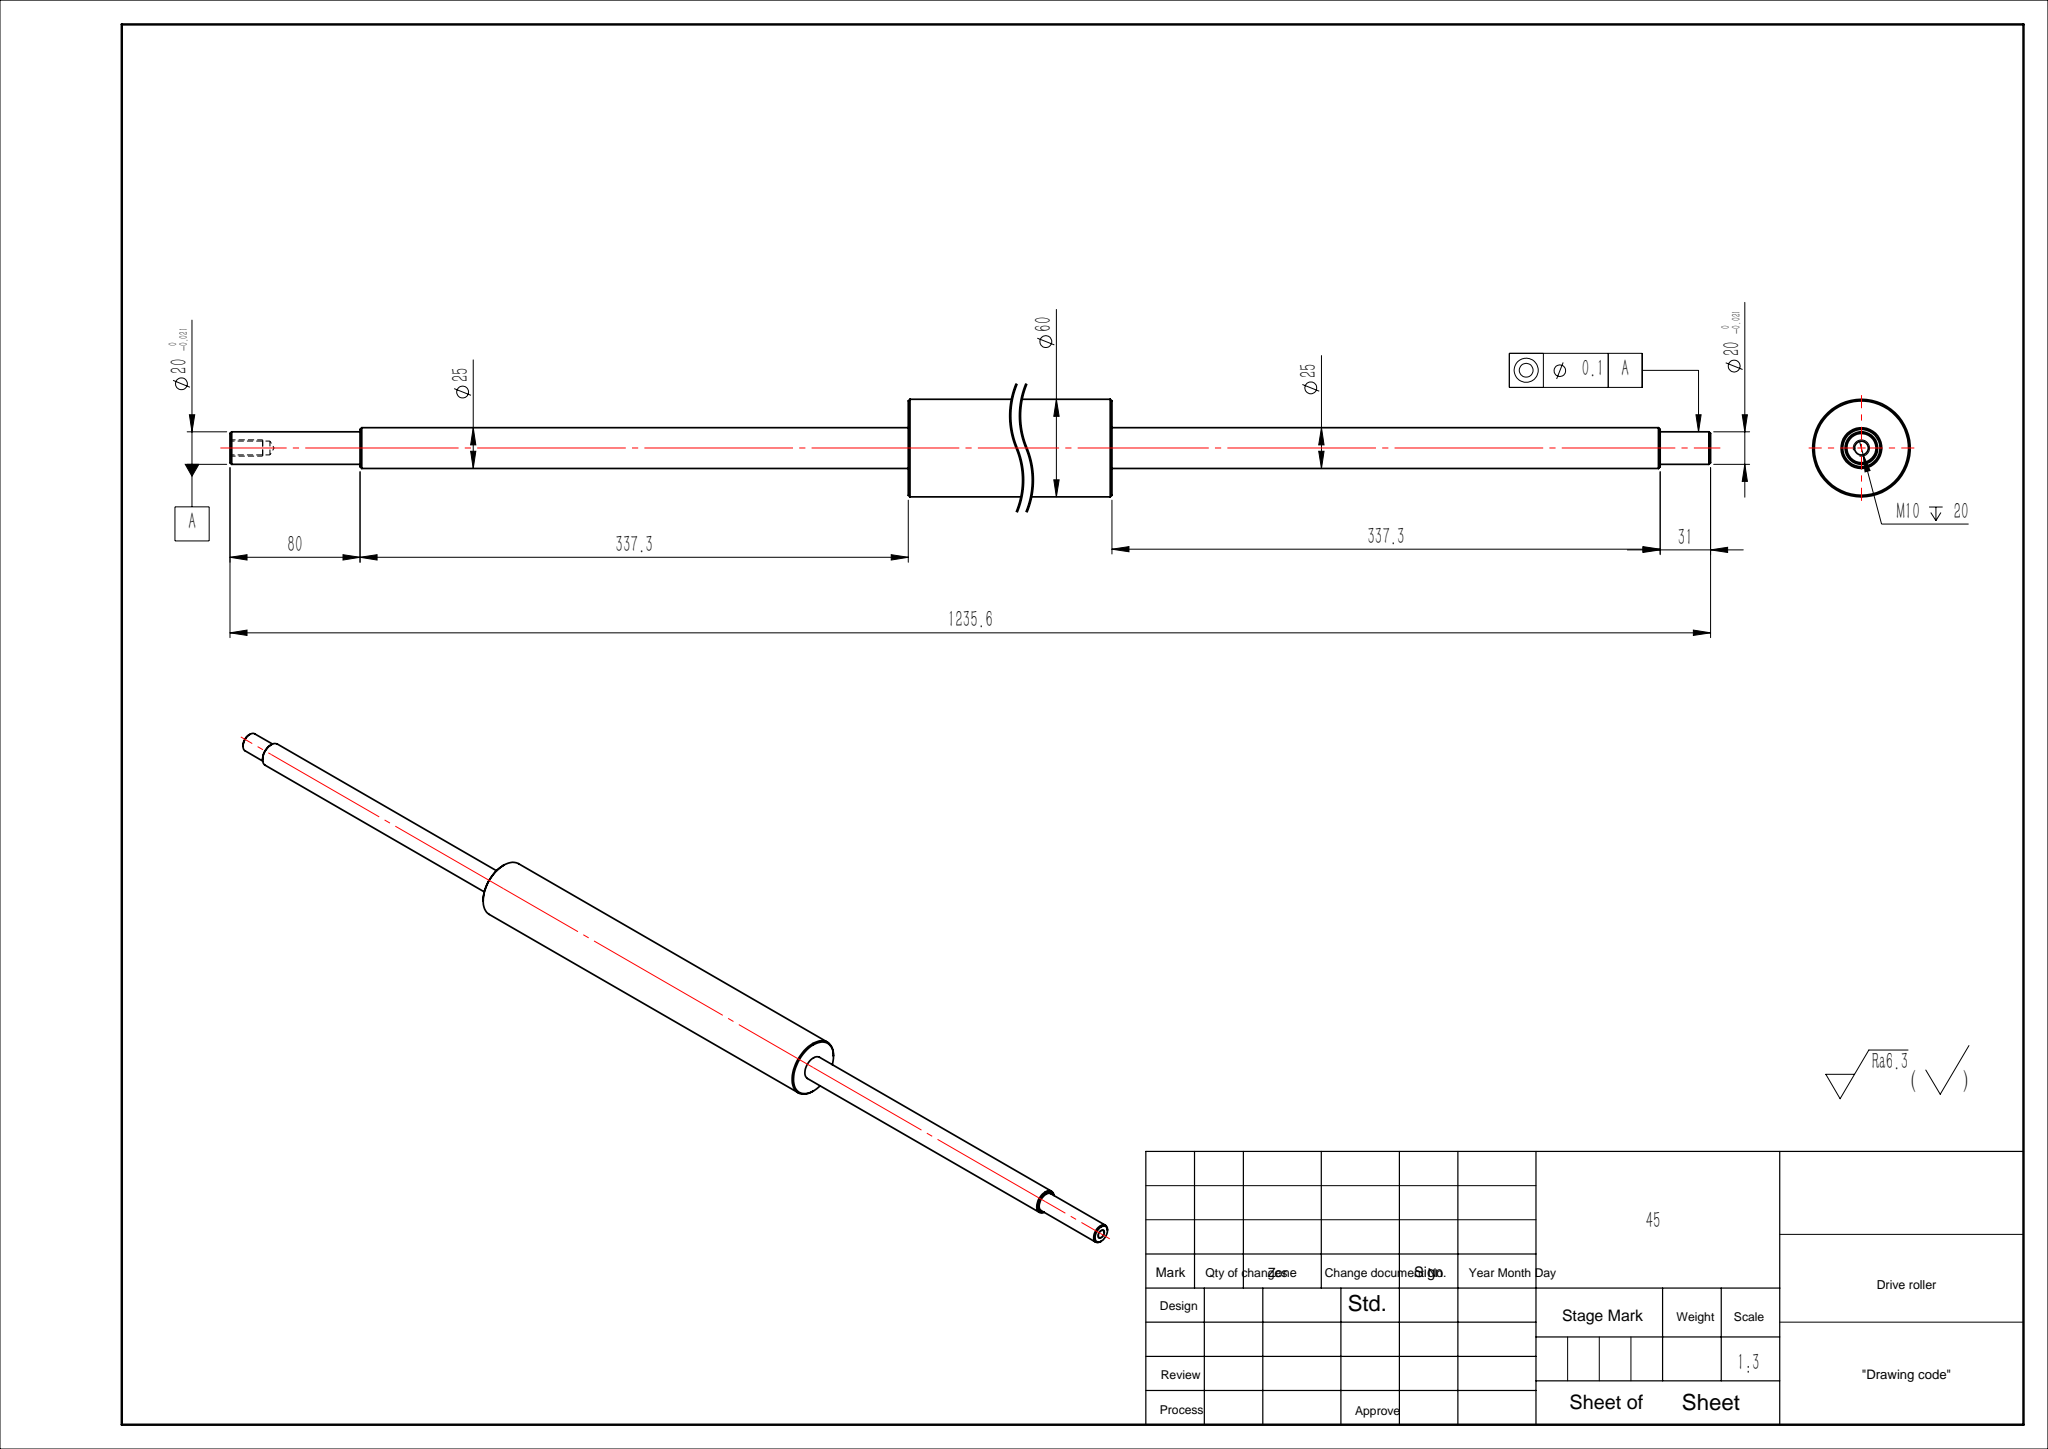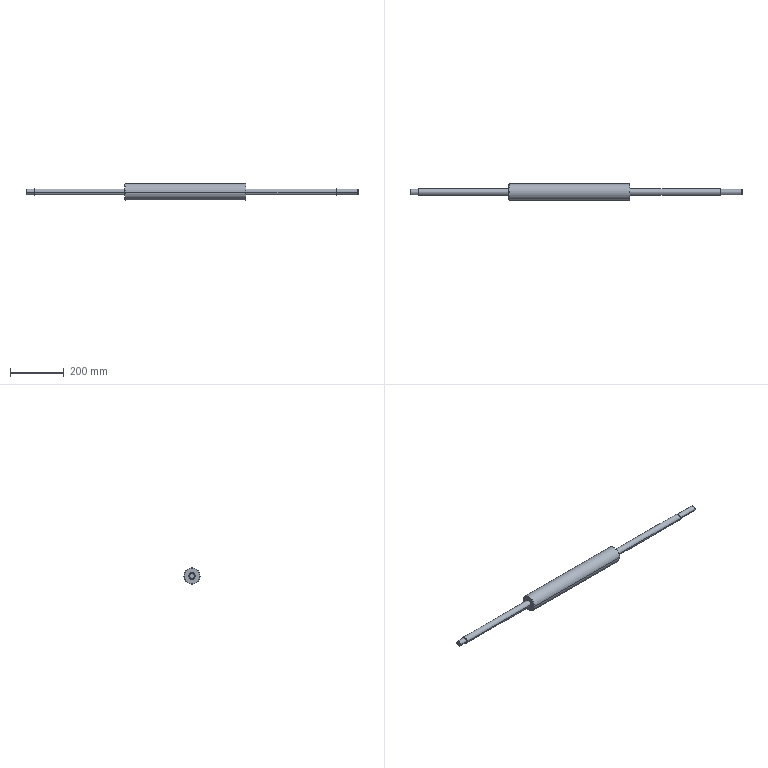Part | SolidWorks | features Chamfer 1, HoleWzd 1, Revolution 1 | 1 solid | 32 faces | box 1236 x 60 x 60 mm | volume 1636598 mm3 | cone 14 | cylinder 12 | plane 6 | commonest cylinder face diameters 20 x4 25 x4 8.5 x2 60 x2
STEP:
#1=CARTESIAN_POINT('',(617.8,0.,4.25));
#2=VERTEX_POINT('',#1);
#3=CARTESIAN_POINT('',(617.8,0.,-4.25));
#4=VERTEX_POINT('',#3);
#5=CARTESIAN_POINT('',(617.8,0.,0.));
#6=DIRECTION('',(1.,0.,0.));
#7=DIRECTION('',(0.,0.,-1.));
#8=AXIS2_PLACEMENT_3D('',#5,#6,#7);
#9=CIRCLE('',#8,4.25);
#10=EDGE_CURVE('',#2,#4,#9,.T.);
#11=ORIENTED_EDGE('',*,*,#10,.F.);
#12=CARTESIAN_POINT('',(642.3,0.,4.25));
#13=VERTEX_POINT('',#12);
#14=CARTESIAN_POINT('',(642.3,0.,4.25));
#15=DIRECTION('',(1.,0.,0.));
#16=VECTOR('',#15,1000.);
#17=LINE('',#14,#16);
#18=EDGE_CURVE('',#2,#13,#17,.T.);
#19=ORIENTED_EDGE('',*,*,#18,.T.);
#20=CARTESIAN_POINT('',(642.3,0.,-4.25));
#21=VERTEX_POINT('',#20);
#22=CARTESIAN_POINT('',(642.3,0.,0.));
#23=DIRECTION('',(1.,0.,0.));
#24=DIRECTION('',(0.,0.,-1.));
#25=AXIS2_PLACEMENT_3D('',#22,#23,#24);
#26=CIRCLE('',#25,4.25);
#27=EDGE_CURVE('',#13,#21,#26,.T.);
#28=ORIENTED_EDGE('',*,*,#27,.T.);
#29=CARTESIAN_POINT('',(642.3,0.,-4.25));
#30=DIRECTION('',(1.,0.,0.));
#31=VECTOR('',#30,1000.);
#32=LINE('',#29,#31);
#33=EDGE_CURVE('',#4,#21,#32,.T.);
#34=ORIENTED_EDGE('',*,*,#33,.F.);
#35=EDGE_LOOP('',(#11,#19,#28,#34));
#36=FACE_OUTER_BOUND('',#35,.T.);
#37=CARTESIAN_POINT('',(642.3,0.,0.));
#38=DIRECTION('',(1.,0.,0.));
#39=DIRECTION('',(0.,0.,-1.));
#40=AXIS2_PLACEMENT_3D('',#37,#38,#39);
#41=CYLINDRICAL_SURFACE('',#40,4.25);
#42=ADVANCED_FACE('',(#36),#41,.F.);
#43=CARTESIAN_POINT('',(615.246,0.,0.));
#44=VERTEX_POINT('',#43);
#45=CARTESIAN_POINT('',(617.8,0.,-4.25));
#46=DIRECTION('',(0.515,0.,-0.8572));
#47=VECTOR('',#46,1000.);
#48=LINE('',#45,#47);
#49=EDGE_CURVE('',#44,#4,#48,.T.);
#50=ORIENTED_EDGE('',*,*,#49,.F.);
#51=CARTESIAN_POINT('',(617.8,0.,4.25));
#52=DIRECTION('',(0.515,0.,0.8572));
#53=VECTOR('',#52,1000.);
#54=LINE('',#51,#53);
#55=EDGE_CURVE('',#44,#2,#54,.T.);
#56=ORIENTED_EDGE('',*,*,#55,.T.);
#57=ORIENTED_EDGE('',*,*,#10,.T.);
#58=EDGE_LOOP('',(#50,#56,#57));
#59=FACE_OUTER_BOUND('',#58,.T.);
#60=CARTESIAN_POINT('',(617.8,0.,0.));
#61=DIRECTION('',(1.,0.,0.));
#62=DIRECTION('',(0.,0.,-1.));
#63=AXIS2_PLACEMENT_3D('',#60,#61,#62);
#64=CONICAL_SURFACE('',#63,4.25,1.03);
#65=ADVANCED_FACE('',(#59),#64,.F.);
#66=CARTESIAN_POINT('',(-593.3,-9.,0.));
#67=VERTEX_POINT('',#66);
#68=CARTESIAN_POINT('',(-593.3,9.,0.));
#69=VERTEX_POINT('',#68);
#70=CARTESIAN_POINT('',(-593.3,0.,0.));
#71=DIRECTION('',(-1.,0.,0.));
#72=DIRECTION('',(0.,-1.,0.));
#73=AXIS2_PLACEMENT_3D('',#70,#71,#72);
#74=CIRCLE('',#73,9.);
#75=EDGE_CURVE('',#67,#69,#74,.T.);
#76=ORIENTED_EDGE('',*,*,#75,.F.);
#77=CARTESIAN_POINT('',(-592.3,-10.,0.));
#78=VERTEX_POINT('',#77);
#79=CARTESIAN_POINT('',(-592.3,-10.,0.));
#80=DIRECTION('',(0.7071,-0.7071,0.));
#81=VECTOR('',#80,1000.);
#82=LINE('',#79,#81);
#83=EDGE_CURVE('',#67,#78,#82,.T.);
#84=ORIENTED_EDGE('',*,*,#83,.T.);
#85=CARTESIAN_POINT('',(-592.3,10.,0.));
#86=VERTEX_POINT('',#85);
#87=CARTESIAN_POINT('',(-592.3,0.,0.));
#88=DIRECTION('',(1.,0.,0.));
#89=DIRECTION('',(0.,-1.,0.));
#90=AXIS2_PLACEMENT_3D('',#87,#88,#89);
#91=CIRCLE('',#90,10.);
#92=EDGE_CURVE('',#86,#78,#91,.T.);
#93=ORIENTED_EDGE('',*,*,#92,.F.);
#94=CARTESIAN_POINT('',(-592.3,10.,0.));
#95=DIRECTION('',(0.7071,0.7071,0.));
#96=VECTOR('',#95,1000.);
#97=LINE('',#94,#96);
#98=EDGE_CURVE('',#69,#86,#97,.T.);
#99=ORIENTED_EDGE('',*,*,#98,.F.);
#100=EDGE_LOOP('',(#76,#84,#93,#99));
#101=FACE_OUTER_BOUND('',#100,.T.);
#102=CARTESIAN_POINT('',(-592.3,0.,0.));
#103=DIRECTION('',(1.,0.,0.));
#104=DIRECTION('',(0.,1.,0.));
#105=AXIS2_PLACEMENT_3D('',#102,#103,#104);
#106=CONICAL_SURFACE('',#105,10.,0.7854);
#107=ADVANCED_FACE('',(#101),#106,.T.);
#108=CARTESIAN_POINT('',(-562.3,-11.5,0.));
#109=VERTEX_POINT('',#108);
#110=CARTESIAN_POINT('',(-562.3,11.5,0.));
#111=VERTEX_POINT('',#110);
#112=CARTESIAN_POINT('',(-562.3,0.,0.));
#113=DIRECTION('',(-1.,0.,0.));
#114=DIRECTION('',(0.,-1.,0.));
#115=AXIS2_PLACEMENT_3D('',#112,#113,#114);
#116=CIRCLE('',#115,11.5);
#117=EDGE_CURVE('',#109,#111,#116,.T.);
#118=ORIENTED_EDGE('',*,*,#117,.F.);
#119=CARTESIAN_POINT('',(-561.3,-12.5,0.));
#120=VERTEX_POINT('',#119);
#121=CARTESIAN_POINT('',(-561.3,-12.5,0.));
#122=DIRECTION('',(0.7071,-0.7071,0.));
#123=VECTOR('',#122,1000.);
#124=LINE('',#121,#123);
#125=EDGE_CURVE('',#109,#120,#124,.T.);
#126=ORIENTED_EDGE('',*,*,#125,.T.);
#127=CARTESIAN_POINT('',(-561.3,12.5,0.));
#128=VERTEX_POINT('',#127);
#129=CARTESIAN_POINT('',(-561.3,0.,0.));
#130=DIRECTION('',(1.,0.,0.));
#131=DIRECTION('',(0.,-1.,0.));
#132=AXIS2_PLACEMENT_3D('',#129,#130,#131);
#133=CIRCLE('',#132,12.5);
#134=EDGE_CURVE('',#128,#120,#133,.T.);
#135=ORIENTED_EDGE('',*,*,#134,.F.);
#136=CARTESIAN_POINT('',(-561.3,12.5,0.));
#137=DIRECTION('',(0.7071,0.7071,0.));
#138=VECTOR('',#137,1000.);
#139=LINE('',#136,#138);
#140=EDGE_CURVE('',#111,#128,#139,.T.);
#141=ORIENTED_EDGE('',*,*,#140,.F.);
#142=EDGE_LOOP('',(#118,#126,#135,#141));
#143=FACE_OUTER_BOUND('',#142,.T.);
#144=CARTESIAN_POINT('',(-561.3,0.,0.));
#145=DIRECTION('',(1.,0.,0.));
#146=DIRECTION('',(0.,1.,0.));
#147=AXIS2_PLACEMENT_3D('',#144,#145,#146);
#148=CONICAL_SURFACE('',#147,12.5,0.7854);
#149=ADVANCED_FACE('',(#143),#148,.T.);
#150=CARTESIAN_POINT('',(-225.,-29.,0.));
#151=VERTEX_POINT('',#150);
#152=CARTESIAN_POINT('',(-225.,29.,0.));
#153=VERTEX_POINT('',#152);
#154=CARTESIAN_POINT('',(-225.,0.,0.));
#155=DIRECTION('',(-1.,0.,0.));
#156=DIRECTION('',(0.,-1.,0.));
#157=AXIS2_PLACEMENT_3D('',#154,#155,#156);
#158=CIRCLE('',#157,29.);
#159=EDGE_CURVE('',#151,#153,#158,.T.);
#160=ORIENTED_EDGE('',*,*,#159,.F.);
#161=CARTESIAN_POINT('',(-224.,-30.,0.));
#162=VERTEX_POINT('',#161);
#163=CARTESIAN_POINT('',(-224.,-30.,0.));
#164=DIRECTION('',(0.7071,-0.7071,0.));
#165=VECTOR('',#164,1000.);
#166=LINE('',#163,#165);
#167=EDGE_CURVE('',#151,#162,#166,.T.);
#168=ORIENTED_EDGE('',*,*,#167,.T.);
#169=CARTESIAN_POINT('',(-224.,30.,0.));
#170=VERTEX_POINT('',#169);
#171=CARTESIAN_POINT('',(-224.,0.,0.));
#172=DIRECTION('',(1.,0.,0.));
#173=DIRECTION('',(0.,-1.,0.));
#174=AXIS2_PLACEMENT_3D('',#171,#172,#173);
#175=CIRCLE('',#174,30.);
#176=EDGE_CURVE('',#170,#162,#175,.T.);
#177=ORIENTED_EDGE('',*,*,#176,.F.);
#178=CARTESIAN_POINT('',(-224.,30.,0.));
#179=DIRECTION('',(0.7071,0.7071,0.));
#180=VECTOR('',#179,1000.);
#181=LINE('',#178,#180);
#182=EDGE_CURVE('',#153,#170,#181,.T.);
#183=ORIENTED_EDGE('',*,*,#182,.F.);
#184=EDGE_LOOP('',(#160,#168,#177,#183));
#185=FACE_OUTER_BOUND('',#184,.T.);
#186=CARTESIAN_POINT('',(-224.,0.,0.));
#187=DIRECTION('',(1.,0.,0.));
#188=DIRECTION('',(0.,1.,0.));
#189=AXIS2_PLACEMENT_3D('',#186,#187,#188);
#190=CONICAL_SURFACE('',#189,30.,0.7854);
#191=ADVANCED_FACE('',(#185),#190,.T.);
#192=CARTESIAN_POINT('',(225.,29.,0.));
#193=VERTEX_POINT('',#192);
#194=CARTESIAN_POINT('',(225.,-29.,0.));
#195=VERTEX_POINT('',#194);
#196=CARTESIAN_POINT('',(225.,0.,0.));
#197=DIRECTION('',(1.,0.,0.));
#198=DIRECTION('',(0.,1.,0.));
#199=AXIS2_PLACEMENT_3D('',#196,#197,#198);
#200=CIRCLE('',#199,29.);
#201=EDGE_CURVE('',#193,#195,#200,.T.);
#202=ORIENTED_EDGE('',*,*,#201,.F.);
#203=CARTESIAN_POINT('',(224.,30.,0.));
#204=VERTEX_POINT('',#203);
#205=CARTESIAN_POINT('',(225.,29.,0.));
#206=DIRECTION('',(-0.7071,0.7071,0.));
#207=VECTOR('',#206,1000.);
#208=LINE('',#205,#207);
#209=EDGE_CURVE('',#193,#204,#208,.T.);
#210=ORIENTED_EDGE('',*,*,#209,.T.);
#211=CARTESIAN_POINT('',(224.,-30.,0.));
#212=VERTEX_POINT('',#211);
#213=CARTESIAN_POINT('',(224.,0.,0.));
#214=DIRECTION('',(-1.,0.,0.));
#215=DIRECTION('',(0.,1.,0.));
#216=AXIS2_PLACEMENT_3D('',#213,#214,#215);
#217=CIRCLE('',#216,30.);
#218=EDGE_CURVE('',#212,#204,#217,.T.);
#219=ORIENTED_EDGE('',*,*,#218,.F.);
#220=CARTESIAN_POINT('',(225.,-29.,0.));
#221=DIRECTION('',(-0.7071,-0.7071,0.));
#222=VECTOR('',#221,1000.);
#223=LINE('',#220,#222);
#224=EDGE_CURVE('',#195,#212,#223,.T.);
#225=ORIENTED_EDGE('',*,*,#224,.F.);
#226=EDGE_LOOP('',(#202,#210,#219,#225));
#227=FACE_OUTER_BOUND('',#226,.T.);
#228=CARTESIAN_POINT('',(225.,0.,0.));
#229=DIRECTION('',(-1.,0.,0.));
#230=DIRECTION('',(0.,-1.,0.));
#231=AXIS2_PLACEMENT_3D('',#228,#229,#230);
#232=CONICAL_SURFACE('',#231,29.,0.7854);
#233=ADVANCED_FACE('',(#227),#232,.T.);
#234=CARTESIAN_POINT('',(562.3,11.5,0.));
#235=VERTEX_POINT('',#234);
#236=CARTESIAN_POINT('',(562.3,-11.5,0.));
#237=VERTEX_POINT('',#236);
#238=CARTESIAN_POINT('',(562.3,0.,0.));
#239=DIRECTION('',(1.,0.,0.));
#240=DIRECTION('',(0.,1.,0.));
#241=AXIS2_PLACEMENT_3D('',#238,#239,#240);
#242=CIRCLE('',#241,11.5);
#243=EDGE_CURVE('',#235,#237,#242,.T.);
#244=ORIENTED_EDGE('',*,*,#243,.F.);
#245=CARTESIAN_POINT('',(561.3,12.5,0.));
#246=VERTEX_POINT('',#245);
#247=CARTESIAN_POINT('',(562.3,11.5,0.));
#248=DIRECTION('',(-0.7071,0.7071,0.));
#249=VECTOR('',#248,1000.);
#250=LINE('',#247,#249);
#251=EDGE_CURVE('',#235,#246,#250,.T.);
#252=ORIENTED_EDGE('',*,*,#251,.T.);
#253=CARTESIAN_POINT('',(561.3,-12.5,0.));
#254=VERTEX_POINT('',#253);
#255=CARTESIAN_POINT('',(561.3,0.,0.));
#256=DIRECTION('',(-1.,0.,0.));
#257=DIRECTION('',(0.,1.,0.));
#258=AXIS2_PLACEMENT_3D('',#255,#256,#257);
#259=CIRCLE('',#258,12.5);
#260=EDGE_CURVE('',#254,#246,#259,.T.);
#261=ORIENTED_EDGE('',*,*,#260,.F.);
#262=CARTESIAN_POINT('',(562.3,-11.5,0.));
#263=DIRECTION('',(-0.7071,-0.7071,0.));
#264=VECTOR('',#263,1000.);
#265=LINE('',#262,#264);
#266=EDGE_CURVE('',#237,#254,#265,.T.);
#267=ORIENTED_EDGE('',*,*,#266,.F.);
#268=EDGE_LOOP('',(#244,#252,#261,#267));
#269=FACE_OUTER_BOUND('',#268,.T.);
#270=CARTESIAN_POINT('',(562.3,0.,0.));
#271=DIRECTION('',(-1.,0.,0.));
#272=DIRECTION('',(0.,-1.,0.));
#273=AXIS2_PLACEMENT_3D('',#270,#271,#272);
#274=CONICAL_SURFACE('',#273,11.5,0.7854);
#275=ADVANCED_FACE('',(#269),#274,.T.);
#276=CARTESIAN_POINT('',(642.3,9.,0.));
#277=VERTEX_POINT('',#276);
#278=CARTESIAN_POINT('',(642.3,-9.,0.));
#279=VERTEX_POINT('',#278);
#280=CARTESIAN_POINT('',(642.3,0.,0.));
#281=DIRECTION('',(1.,0.,0.));
#282=DIRECTION('',(0.,1.,0.));
#283=AXIS2_PLACEMENT_3D('',#280,#281,#282);
#284=CIRCLE('',#283,9.);
#285=EDGE_CURVE('',#277,#279,#284,.T.);
#286=ORIENTED_EDGE('',*,*,#285,.F.);
#287=CARTESIAN_POINT('',(641.3,10.,0.));
#288=VERTEX_POINT('',#287);
#289=CARTESIAN_POINT('',(642.3,9.,0.));
#290=DIRECTION('',(-0.7071,0.7071,0.));
#291=VECTOR('',#290,1000.);
#292=LINE('',#289,#291);
#293=EDGE_CURVE('',#277,#288,#292,.T.);
#294=ORIENTED_EDGE('',*,*,#293,.T.);
#295=CARTESIAN_POINT('',(641.3,-10.,0.));
#296=VERTEX_POINT('',#295);
#297=CARTESIAN_POINT('',(641.3,0.,0.));
#298=DIRECTION('',(-1.,0.,0.));
#299=DIRECTION('',(0.,1.,0.));
#300=AXIS2_PLACEMENT_3D('',#297,#298,#299);
#301=CIRCLE('',#300,10.);
#302=EDGE_CURVE('',#296,#288,#301,.T.);
#303=ORIENTED_EDGE('',*,*,#302,.F.);
#304=CARTESIAN_POINT('',(642.3,-9.,0.));
#305=DIRECTION('',(-0.7071,-0.7071,0.));
#306=VECTOR('',#305,1000.);
#307=LINE('',#304,#306);
#308=EDGE_CURVE('',#279,#296,#307,.T.);
#309=ORIENTED_EDGE('',*,*,#308,.F.);
#310=EDGE_LOOP('',(#286,#294,#303,#309));
#311=FACE_OUTER_BOUND('',#310,.T.);
#312=CARTESIAN_POINT('',(642.3,0.,0.));
#313=DIRECTION('',(-1.,0.,0.));
#314=DIRECTION('',(0.,-1.,0.));
#315=AXIS2_PLACEMENT_3D('',#312,#313,#314);
#316=CONICAL_SURFACE('',#315,9.,0.7854);
#317=ADVANCED_FACE('',(#311),#316,.T.);
#318=CARTESIAN_POINT('',(562.3,10.,0.));
#319=VERTEX_POINT('',#318);
#320=CARTESIAN_POINT('',(562.3,-10.,0.));
#321=VERTEX_POINT('',#320);
#322=CARTESIAN_POINT('',(562.3,0.,0.));
#323=DIRECTION('',(1.,0.,0.));
#324=DIRECTION('',(0.,1.,0.));
#325=AXIS2_PLACEMENT_3D('',#322,#323,#324);
#326=CIRCLE('',#325,10.);
#327=EDGE_CURVE('',#319,#321,#326,.T.);
#328=ORIENTED_EDGE('',*,*,#327,.T.);
#329=CARTESIAN_POINT('',(642.3,-10.,0.));
#330=DIRECTION('',(1.,0.,0.));
#331=VECTOR('',#330,1000.);
#332=LINE('',#329,#331);
#333=EDGE_CURVE('',#321,#296,#332,.T.);
#334=ORIENTED_EDGE('',*,*,#333,.T.);
#335=ORIENTED_EDGE('',*,*,#302,.T.);
#336=CARTESIAN_POINT('',(642.3,10.,0.));
#337=DIRECTION('',(1.,0.,0.));
#338=VECTOR('',#337,1000.);
#339=LINE('',#336,#338);
#340=EDGE_CURVE('',#319,#288,#339,.T.);
#341=ORIENTED_EDGE('',*,*,#340,.F.);
#342=EDGE_LOOP('',(#328,#334,#335,#341));
#343=FACE_OUTER_BOUND('',#342,.T.);
#344=CARTESIAN_POINT('',(642.3,0.,0.));
#345=DIRECTION('',(1.,0.,0.));
#346=DIRECTION('',(0.,1.,0.));
#347=AXIS2_PLACEMENT_3D('',#344,#345,#346);
#348=CYLINDRICAL_SURFACE('',#347,10.);
#349=ADVANCED_FACE('',(#343),#348,.T.);
#350=CARTESIAN_POINT('',(225.,12.5,0.));
#351=VERTEX_POINT('',#350);
#352=CARTESIAN_POINT('',(225.,-12.5,0.));
#353=VERTEX_POINT('',#352);
#354=CARTESIAN_POINT('',(225.,0.,0.));
#355=DIRECTION('',(1.,0.,0.));
#356=DIRECTION('',(0.,1.,0.));
#357=AXIS2_PLACEMENT_3D('',#354,#355,#356);
#358=CIRCLE('',#357,12.5);
#359=EDGE_CURVE('',#351,#353,#358,.T.);
#360=ORIENTED_EDGE('',*,*,#359,.T.);
#361=CARTESIAN_POINT('',(642.3,-12.5,0.));
#362=DIRECTION('',(1.,0.,0.));
#363=VECTOR('',#362,1000.);
#364=LINE('',#361,#363);
#365=EDGE_CURVE('',#353,#254,#364,.T.);
#366=ORIENTED_EDGE('',*,*,#365,.T.);
#367=ORIENTED_EDGE('',*,*,#260,.T.);
#368=CARTESIAN_POINT('',(642.3,12.5,0.));
#369=DIRECTION('',(1.,0.,0.));
#370=VECTOR('',#369,1000.);
#371=LINE('',#368,#370);
#372=EDGE_CURVE('',#351,#246,#371,.T.);
#373=ORIENTED_EDGE('',*,*,#372,.F.);
#374=EDGE_LOOP('',(#360,#366,#367,#373));
#375=FACE_OUTER_BOUND('',#374,.T.);
#376=CARTESIAN_POINT('',(642.3,0.,0.));
#377=DIRECTION('',(1.,0.,0.));
#378=DIRECTION('',(0.,1.,0.));
#379=AXIS2_PLACEMENT_3D('',#376,#377,#378);
#380=CYLINDRICAL_SURFACE('',#379,12.5);
#381=ADVANCED_FACE('',(#375),#380,.T.);
#382=ORIENTED_EDGE('',*,*,#176,.T.);
#383=CARTESIAN_POINT('',(642.3,-30.,0.));
#384=DIRECTION('',(1.,0.,0.));
#385=VECTOR('',#384,1000.);
#386=LINE('',#383,#385);
#387=EDGE_CURVE('',#162,#212,#386,.T.);
#388=ORIENTED_EDGE('',*,*,#387,.T.);
#389=ORIENTED_EDGE('',*,*,#218,.T.);
#390=CARTESIAN_POINT('',(642.3,30.,0.));
#391=DIRECTION('',(1.,0.,0.));
#392=VECTOR('',#391,1000.);
#393=LINE('',#390,#392);
#394=EDGE_CURVE('',#170,#204,#393,.T.);
#395=ORIENTED_EDGE('',*,*,#394,.F.);
#396=EDGE_LOOP('',(#382,#388,#389,#395));
#397=FACE_OUTER_BOUND('',#396,.T.);
#398=CARTESIAN_POINT('',(642.3,0.,0.));
#399=DIRECTION('',(1.,0.,0.));
#400=DIRECTION('',(0.,1.,0.));
#401=AXIS2_PLACEMENT_3D('',#398,#399,#400);
#402=CYLINDRICAL_SURFACE('',#401,30.);
#403=ADVANCED_FACE('',(#397),#402,.T.);
#404=ORIENTED_EDGE('',*,*,#134,.T.);
#405=CARTESIAN_POINT('',(-225.,-12.5,0.));
#406=VERTEX_POINT('',#405);
#407=CARTESIAN_POINT('',(642.3,-12.5,0.));
#408=DIRECTION('',(1.,0.,0.));
#409=VECTOR('',#408,1000.);
#410=LINE('',#407,#409);
#411=EDGE_CURVE('',#120,#406,#410,.T.);
#412=ORIENTED_EDGE('',*,*,#411,.T.);
#413=CARTESIAN_POINT('',(-225.,12.5,0.));
#414=VERTEX_POINT('',#413);
#415=CARTESIAN_POINT('',(-225.,0.,0.));
#416=DIRECTION('',(1.,0.,0.));
#417=DIRECTION('',(0.,1.,0.));
#418=AXIS2_PLACEMENT_3D('',#415,#416,#417);
#419=CIRCLE('',#418,12.5);
#420=EDGE_CURVE('',#414,#406,#419,.T.);
#421=ORIENTED_EDGE('',*,*,#420,.F.);
#422=CARTESIAN_POINT('',(642.3,12.5,0.));
#423=DIRECTION('',(1.,0.,0.));
#424=VECTOR('',#423,1000.);
#425=LINE('',#422,#424);
#426=EDGE_CURVE('',#128,#414,#425,.T.);
#427=ORIENTED_EDGE('',*,*,#426,.F.);
#428=EDGE_LOOP('',(#404,#412,#421,#427));
#429=FACE_OUTER_BOUND('',#428,.T.);
#430=CARTESIAN_POINT('',(642.3,0.,0.));
#431=DIRECTION('',(1.,0.,0.));
#432=DIRECTION('',(0.,1.,0.));
#433=AXIS2_PLACEMENT_3D('',#430,#431,#432);
#434=CYLINDRICAL_SURFACE('',#433,12.5);
#435=ADVANCED_FACE('',(#429),#434,.T.);
#436=ORIENTED_EDGE('',*,*,#92,.T.);
#437=CARTESIAN_POINT('',(-562.3,-10.,0.));
#438=VERTEX_POINT('',#437);
#439=CARTESIAN_POINT('',(642.3,-10.,0.));
#440=DIRECTION('',(1.,0.,0.));
#441=VECTOR('',#440,1000.);
#442=LINE('',#439,#441);
#443=EDGE_CURVE('',#78,#438,#442,.T.);
#444=ORIENTED_EDGE('',*,*,#443,.T.);
#445=CARTESIAN_POINT('',(-562.3,10.,0.));
#446=VERTEX_POINT('',#445);
#447=CARTESIAN_POINT('',(-562.3,0.,0.));
#448=DIRECTION('',(1.,0.,0.));
#449=DIRECTION('',(0.,1.,0.));
#450=AXIS2_PLACEMENT_3D('',#447,#448,#449);
#451=CIRCLE('',#450,10.);
#452=EDGE_CURVE('',#446,#438,#451,.T.);
#453=ORIENTED_EDGE('',*,*,#452,.F.);
#454=CARTESIAN_POINT('',(642.3,10.,0.));
#455=DIRECTION('',(1.,0.,0.));
#456=VECTOR('',#455,1000.);
#457=LINE('',#454,#456);
#458=EDGE_CURVE('',#86,#446,#457,.T.);
#459=ORIENTED_EDGE('',*,*,#458,.F.);
#460=EDGE_LOOP('',(#436,#444,#453,#459));
#461=FACE_OUTER_BOUND('',#460,.T.);
#462=CARTESIAN_POINT('',(642.3,0.,0.));
#463=DIRECTION('',(1.,0.,0.));
#464=DIRECTION('',(0.,1.,0.));
#465=AXIS2_PLACEMENT_3D('',#462,#463,#464);
#466=CYLINDRICAL_SURFACE('',#465,10.);
#467=ADVANCED_FACE('',(#461),#466,.T.);
#468=CARTESIAN_POINT('',(-593.3,0.,0.));
#469=DIRECTION('',(-1.,0.,0.));
#470=DIRECTION('',(0.,-1.,0.));
#471=AXIS2_PLACEMENT_3D('',#468,#469,#470);
#472=CIRCLE('',#471,9.);
#473=EDGE_CURVE('',#69,#67,#472,.T.);
#474=ORIENTED_EDGE('',*,*,#473,.T.);
#475=ORIENTED_EDGE('',*,*,#75,.T.);
#476=EDGE_LOOP('',(#474,#475));
#477=FACE_OUTER_BOUND('',#476,.T.);
#478=CARTESIAN_POINT('',(-593.3,0.,0.));
#479=DIRECTION('',(-1.,0.,0.));
#480=DIRECTION('',(0.,-1.,0.));
#481=AXIS2_PLACEMENT_3D('',#478,#479,#480);
#482=PLANE('',#481);
#483=ADVANCED_FACE('',(#477),#482,.T.);
#484=ORIENTED_EDGE('',*,*,#443,.F.);
#485=CARTESIAN_POINT('',(-592.3,0.,0.));
#486=DIRECTION('',(1.,0.,0.));
#487=DIRECTION('',(0.,-1.,0.));
#488=AXIS2_PLACEMENT_3D('',#485,#486,#487);
#489=CIRCLE('',#488,10.);
#490=EDGE_CURVE('',#78,#86,#489,.T.);
#491=ORIENTED_EDGE('',*,*,#490,.T.);
#492=ORIENTED_EDGE('',*,*,#458,.T.);
#493=CARTESIAN_POINT('',(-562.3,0.,0.));
#494=DIRECTION('',(1.,0.,0.));
#495=DIRECTION('',(0.,1.,0.));
#496=AXIS2_PLACEMENT_3D('',#493,#494,#495);
#497=CIRCLE('',#496,10.);
#498=EDGE_CURVE('',#438,#446,#497,.T.);
#499=ORIENTED_EDGE('',*,*,#498,.F.);
#500=EDGE_LOOP('',(#484,#491,#492,#499));
#501=FACE_OUTER_BOUND('',#500,.T.);
#502=CARTESIAN_POINT('',(642.3,0.,0.));
#503=DIRECTION('',(1.,0.,0.));
#504=DIRECTION('',(0.,1.,0.));
#505=AXIS2_PLACEMENT_3D('',#502,#503,#504);
#506=CYLINDRICAL_SURFACE('',#505,10.);
#507=ADVANCED_FACE('',(#501),#506,.T.);
#508=CARTESIAN_POINT('',(-562.3,0.,0.));
#509=DIRECTION('',(-1.,0.,0.));
#510=DIRECTION('',(0.,-1.,0.));
#511=AXIS2_PLACEMENT_3D('',#508,#509,#510);
#512=CIRCLE('',#511,11.5);
#513=EDGE_CURVE('',#111,#109,#512,.T.);
#514=ORIENTED_EDGE('',*,*,#513,.T.);
#515=ORIENTED_EDGE('',*,*,#117,.T.);
#516=EDGE_LOOP('',(#514,#515));
#517=FACE_OUTER_BOUND('',#516,.T.);
#518=ORIENTED_EDGE('',*,*,#452,.T.);
#519=ORIENTED_EDGE('',*,*,#498,.T.);
#520=EDGE_LOOP('',(#518,#519));
#521=FACE_BOUND('',#520,.T.);
#522=CARTESIAN_POINT('',(-562.3,10.,0.));
#523=DIRECTION('',(-1.,0.,0.));
#524=DIRECTION('',(0.,-1.,0.));
#525=AXIS2_PLACEMENT_3D('',#522,#523,#524);
#526=PLANE('',#525);
#527=ADVANCED_FACE('',(#517,#521),#526,.T.);
#528=ORIENTED_EDGE('',*,*,#411,.F.);
#529=CARTESIAN_POINT('',(-561.3,0.,0.));
#530=DIRECTION('',(1.,0.,0.));
#531=DIRECTION('',(0.,-1.,0.));
#532=AXIS2_PLACEMENT_3D('',#529,#530,#531);
#533=CIRCLE('',#532,12.5);
#534=EDGE_CURVE('',#120,#128,#533,.T.);
#535=ORIENTED_EDGE('',*,*,#534,.T.);
#536=ORIENTED_EDGE('',*,*,#426,.T.);
#537=CARTESIAN_POINT('',(-225.,0.,0.));
#538=DIRECTION('',(1.,0.,0.));
#539=DIRECTION('',(0.,1.,0.));
#540=AXIS2_PLACEMENT_3D('',#537,#538,#539);
#541=CIRCLE('',#540,12.5);
#542=EDGE_CURVE('',#406,#414,#541,.T.);
#543=ORIENTED_EDGE('',*,*,#542,.F.);
#544=EDGE_LOOP('',(#528,#535,#536,#543));
#545=FACE_OUTER_BOUND('',#544,.T.);
#546=CARTESIAN_POINT('',(642.3,0.,0.));
#547=DIRECTION('',(1.,0.,0.));
#548=DIRECTION('',(0.,1.,0.));
#549=AXIS2_PLACEMENT_3D('',#546,#547,#548);
#550=CYLINDRICAL_SURFACE('',#549,12.5);
#551=ADVANCED_FACE('',(#545),#550,.T.);
#552=CARTESIAN_POINT('',(-225.,0.,0.));
#553=DIRECTION('',(-1.,0.,0.));
#554=DIRECTION('',(0.,-1.,0.));
#555=AXIS2_PLACEMENT_3D('',#552,#553,#554);
#556=CIRCLE('',#555,29.);
#557=EDGE_CURVE('',#153,#151,#556,.T.);
#558=ORIENTED_EDGE('',*,*,#557,.T.);
#559=ORIENTED_EDGE('',*,*,#159,.T.);
#560=EDGE_LOOP('',(#558,#559));
#561=FACE_OUTER_BOUND('',#560,.T.);
#562=ORIENTED_EDGE('',*,*,#420,.T.);
#563=ORIENTED_EDGE('',*,*,#542,.T.);
#564=EDGE_LOOP('',(#562,#563));
#565=FACE_BOUND('',#564,.T.);
#566=CARTESIAN_POINT('',(-225.,12.5,0.));
#567=DIRECTION('',(-1.,0.,0.));
#568=DIRECTION('',(0.,-1.,0.));
#569=AXIS2_PLACEMENT_3D('',#566,#567,#568);
#570=PLANE('',#569);
#571=ADVANCED_FACE('',(#561,#565),#570,.T.);
#572=ORIENTED_EDGE('',*,*,#387,.F.);
#573=CARTESIAN_POINT('',(-224.,0.,0.));
#574=DIRECTION('',(1.,0.,0.));
#575=DIRECTION('',(0.,-1.,0.));
#576=AXIS2_PLACEMENT_3D('',#573,#574,#575);
#577=CIRCLE('',#576,30.);
#578=EDGE_CURVE('',#162,#170,#577,.T.);
#579=ORIENTED_EDGE('',*,*,#578,.T.);
#580=ORIENTED_EDGE('',*,*,#394,.T.);
#581=CARTESIAN_POINT('',(224.,0.,0.));
#582=DIRECTION('',(-1.,0.,0.));
#583=DIRECTION('',(0.,1.,0.));
#584=AXIS2_PLACEMENT_3D('',#581,#582,#583);
#585=CIRCLE('',#584,30.);
#586=EDGE_CURVE('',#204,#212,#585,.T.);
#587=ORIENTED_EDGE('',*,*,#586,.T.);
#588=EDGE_LOOP('',(#572,#579,#580,#587));
#589=FACE_OUTER_BOUND('',#588,.T.);
#590=CARTESIAN_POINT('',(642.3,0.,0.));
#591=DIRECTION('',(1.,0.,0.));
#592=DIRECTION('',(0.,1.,0.));
#593=AXIS2_PLACEMENT_3D('',#590,#591,#592);
#594=CYLINDRICAL_SURFACE('',#593,30.);
#595=ADVANCED_FACE('',(#589),#594,.T.);
#596=CARTESIAN_POINT('',(225.,0.,0.));
#597=DIRECTION('',(1.,0.,0.));
#598=DIRECTION('',(0.,1.,0.));
#599=AXIS2_PLACEMENT_3D('',#596,#597,#598);
#600=CIRCLE('',#599,29.);
#601=EDGE_CURVE('',#195,#193,#600,.T.);
#602=ORIENTED_EDGE('',*,*,#601,.T.);
#603=ORIENTED_EDGE('',*,*,#201,.T.);
#604=EDGE_LOOP('',(#602,#603));
#605=FACE_OUTER_BOUND('',#604,.T.);
#606=ORIENTED_EDGE('',*,*,#359,.F.);
#607=CARTESIAN_POINT('',(225.,0.,0.));
#608=DIRECTION('',(1.,0.,0.));
#609=DIRECTION('',(0.,1.,0.));
#610=AXIS2_PLACEMENT_3D('',#607,#608,#609);
#611=CIRCLE('',#610,12.5);
#612=EDGE_CURVE('',#353,#351,#611,.T.);
#613=ORIENTED_EDGE('',*,*,#612,.F.);
#614=EDGE_LOOP('',(#606,#613));
#615=FACE_BOUND('',#614,.T.);
#616=CARTESIAN_POINT('',(225.,30.,0.));
#617=DIRECTION('',(1.,0.,0.));
#618=DIRECTION('',(0.,1.,0.));
#619=AXIS2_PLACEMENT_3D('',#616,#617,#618);
#620=PLANE('',#619);
#621=ADVANCED_FACE('',(#605,#615),#620,.T.);
#622=ORIENTED_EDGE('',*,*,#365,.F.);
#623=ORIENTED_EDGE('',*,*,#612,.T.);
#624=ORIENTED_EDGE('',*,*,#372,.T.);
#625=CARTESIAN_POINT('',(561.3,0.,0.));
#626=DIRECTION('',(-1.,0.,0.));
#627=DIRECTION('',(0.,1.,0.));
#628=AXIS2_PLACEMENT_3D('',#625,#626,#627);
#629=CIRCLE('',#628,12.5);
#630=EDGE_CURVE('',#246,#254,#629,.T.);
#631=ORIENTED_EDGE('',*,*,#630,.T.);
#632=EDGE_LOOP('',(#622,#623,#624,#631));
#633=FACE_OUTER_BOUND('',#632,.T.);
#634=CARTESIAN_POINT('',(642.3,0.,0.));
#635=DIRECTION('',(1.,0.,0.));
#636=DIRECTION('',(0.,1.,0.));
#637=AXIS2_PLACEMENT_3D('',#634,#635,#636);
#638=CYLINDRICAL_SURFACE('',#637,12.5);
#639=ADVANCED_FACE('',(#633),#638,.T.);
#640=CARTESIAN_POINT('',(562.3,0.,0.));
#641=DIRECTION('',(1.,0.,0.));
#642=DIRECTION('',(0.,1.,0.));
#643=AXIS2_PLACEMENT_3D('',#640,#641,#642);
#644=CIRCLE('',#643,11.5);
#645=EDGE_CURVE('',#237,#235,#644,.T.);
#646=ORIENTED_EDGE('',*,*,#645,.T.);
#647=ORIENTED_EDGE('',*,*,#243,.T.);
#648=EDGE_LOOP('',(#646,#647));
#649=FACE_OUTER_BOUND('',#648,.T.);
#650=ORIENTED_EDGE('',*,*,#327,.F.);
#651=CARTESIAN_POINT('',(562.3,0.,0.));
#652=DIRECTION('',(1.,0.,0.));
#653=DIRECTION('',(0.,1.,0.));
#654=AXIS2_PLACEMENT_3D('',#651,#652,#653);
#655=CIRCLE('',#654,10.);
#656=EDGE_CURVE('',#321,#319,#655,.T.);
#657=ORIENTED_EDGE('',*,*,#656,.F.);
#658=EDGE_LOOP('',(#650,#657));
#659=FACE_BOUND('',#658,.T.);
#660=CARTESIAN_POINT('',(562.3,12.5,0.));
#661=DIRECTION('',(1.,0.,0.));
#662=DIRECTION('',(0.,1.,0.));
#663=AXIS2_PLACEMENT_3D('',#660,#661,#662);
#664=PLANE('',#663);
#665=ADVANCED_FACE('',(#649,#659),#664,.T.);
#666=ORIENTED_EDGE('',*,*,#333,.F.);
#667=ORIENTED_EDGE('',*,*,#656,.T.);
#668=ORIENTED_EDGE('',*,*,#340,.T.);
#669=CARTESIAN_POINT('',(641.3,0.,0.));
#670=DIRECTION('',(-1.,0.,0.));
#671=DIRECTION('',(0.,1.,0.));
#672=AXIS2_PLACEMENT_3D('',#669,#670,#671);
#673=CIRCLE('',#672,10.);
#674=EDGE_CURVE('',#288,#296,#673,.T.);
#675=ORIENTED_EDGE('',*,*,#674,.T.);
#676=EDGE_LOOP('',(#666,#667,#668,#675));
#677=FACE_OUTER_BOUND('',#676,.T.);
#678=CARTESIAN_POINT('',(642.3,0.,0.));
#679=DIRECTION('',(1.,0.,0.));
#680=DIRECTION('',(0.,1.,0.));
#681=AXIS2_PLACEMENT_3D('',#678,#679,#680);
#682=CYLINDRICAL_SURFACE('',#681,10.);
#683=ADVANCED_FACE('',(#677),#682,.T.);
#684=CARTESIAN_POINT('',(642.3,0.,0.));
#685=DIRECTION('',(1.,0.,0.));
#686=DIRECTION('',(0.,0.,-1.));
#687=AXIS2_PLACEMENT_3D('',#684,#685,#686);
#688=CIRCLE('',#687,4.25);
#689=EDGE_CURVE('',#21,#13,#688,.T.);
#690=ORIENTED_EDGE('',*,*,#689,.F.);
#691=ORIENTED_EDGE('',*,*,#27,.F.);
#692=EDGE_LOOP('',(#690,#691));
#693=FACE_BOUND('',#692,.T.);
#694=CARTESIAN_POINT('',(642.3,0.,0.));
#695=DIRECTION('',(1.,0.,0.));
#696=DIRECTION('',(0.,1.,0.));
#697=AXIS2_PLACEMENT_3D('',#694,#695,#696);
#698=CIRCLE('',#697,9.);
#699=EDGE_CURVE('',#279,#277,#698,.T.);
#700=ORIENTED_EDGE('',*,*,#699,.T.);
#701=ORIENTED_EDGE('',*,*,#285,.T.);
#702=EDGE_LOOP('',(#700,#701));
#703=FACE_OUTER_BOUND('',#702,.T.);
#704=CARTESIAN_POINT('',(642.3,10.,0.));
#705=DIRECTION('',(1.,0.,0.));
#706=DIRECTION('',(0.,1.,0.));
#707=AXIS2_PLACEMENT_3D('',#704,#705,#706);
#708=PLANE('',#707);
#709=ADVANCED_FACE('',(#693,#703),#708,.T.);
#710=ORIENTED_EDGE('',*,*,#293,.F.);
#711=ORIENTED_EDGE('',*,*,#699,.F.);
#712=ORIENTED_EDGE('',*,*,#308,.T.);
#713=ORIENTED_EDGE('',*,*,#674,.F.);
#714=EDGE_LOOP('',(#710,#711,#712,#713));
#715=FACE_OUTER_BOUND('',#714,.T.);
#716=CARTESIAN_POINT('',(642.3,0.,0.));
#717=DIRECTION('',(-1.,0.,0.));
#718=DIRECTION('',(0.,-1.,0.));
#719=AXIS2_PLACEMENT_3D('',#716,#717,#718);
#720=CONICAL_SURFACE('',#719,9.,0.7854);
#721=ADVANCED_FACE('',(#715),#720,.T.);
#722=ORIENTED_EDGE('',*,*,#251,.F.);
#723=ORIENTED_EDGE('',*,*,#645,.F.);
#724=ORIENTED_EDGE('',*,*,#266,.T.);
#725=ORIENTED_EDGE('',*,*,#630,.F.);
#726=EDGE_LOOP('',(#722,#723,#724,#725));
#727=FACE_OUTER_BOUND('',#726,.T.);
#728=CARTESIAN_POINT('',(562.3,0.,0.));
#729=DIRECTION('',(-1.,0.,0.));
#730=DIRECTION('',(0.,-1.,0.));
#731=AXIS2_PLACEMENT_3D('',#728,#729,#730);
#732=CONICAL_SURFACE('',#731,11.5,0.7854);
#733=ADVANCED_FACE('',(#727),#732,.T.);
#734=ORIENTED_EDGE('',*,*,#209,.F.);
#735=ORIENTED_EDGE('',*,*,#601,.F.);
#736=ORIENTED_EDGE('',*,*,#224,.T.);
#737=ORIENTED_EDGE('',*,*,#586,.F.);
#738=EDGE_LOOP('',(#734,#735,#736,#737));
#739=FACE_OUTER_BOUND('',#738,.T.);
#740=CARTESIAN_POINT('',(225.,0.,0.));
#741=DIRECTION('',(-1.,0.,0.));
#742=DIRECTION('',(0.,-1.,0.));
#743=AXIS2_PLACEMENT_3D('',#740,#741,#742);
#744=CONICAL_SURFACE('',#743,29.,0.7854);
#745=ADVANCED_FACE('',(#739),#744,.T.);
#746=ORIENTED_EDGE('',*,*,#167,.F.);
#747=ORIENTED_EDGE('',*,*,#557,.F.);
#748=ORIENTED_EDGE('',*,*,#182,.T.);
#749=ORIENTED_EDGE('',*,*,#578,.F.);
#750=EDGE_LOOP('',(#746,#747,#748,#749));
#751=FACE_OUTER_BOUND('',#750,.T.);
#752=CARTESIAN_POINT('',(-224.,0.,0.));
#753=DIRECTION('',(1.,0.,0.));
#754=DIRECTION('',(0.,1.,0.));
#755=AXIS2_PLACEMENT_3D('',#752,#753,#754);
#756=CONICAL_SURFACE('',#755,30.,0.7854);
#757=ADVANCED_FACE('',(#751),#756,.T.);
#758=ORIENTED_EDGE('',*,*,#125,.F.);
#759=ORIENTED_EDGE('',*,*,#513,.F.);
#760=ORIENTED_EDGE('',*,*,#140,.T.);
#761=ORIENTED_EDGE('',*,*,#534,.F.);
#762=EDGE_LOOP('',(#758,#759,#760,#761));
#763=FACE_OUTER_BOUND('',#762,.T.);
#764=CARTESIAN_POINT('',(-561.3,0.,0.));
#765=DIRECTION('',(1.,0.,0.));
#766=DIRECTION('',(0.,1.,0.));
#767=AXIS2_PLACEMENT_3D('',#764,#765,#766);
#768=CONICAL_SURFACE('',#767,12.5,0.7854);
#769=ADVANCED_FACE('',(#763),#768,.T.);
#770=ORIENTED_EDGE('',*,*,#83,.F.);
#771=ORIENTED_EDGE('',*,*,#473,.F.);
#772=ORIENTED_EDGE('',*,*,#98,.T.);
#773=ORIENTED_EDGE('',*,*,#490,.F.);
#774=EDGE_LOOP('',(#770,#771,#772,#773));
#775=FACE_OUTER_BOUND('',#774,.T.);
#776=CARTESIAN_POINT('',(-592.3,0.,0.));
#777=DIRECTION('',(1.,0.,0.));
#778=DIRECTION('',(0.,1.,0.));
#779=AXIS2_PLACEMENT_3D('',#776,#777,#778);
#780=CONICAL_SURFACE('',#779,10.,0.7854);
#781=ADVANCED_FACE('',(#775),#780,.T.);
#782=ORIENTED_EDGE('',*,*,#55,.F.);
#783=ORIENTED_EDGE('',*,*,#49,.T.);
#784=CARTESIAN_POINT('',(617.8,0.,0.));
#785=DIRECTION('',(1.,0.,0.));
#786=DIRECTION('',(0.,0.,-1.));
#787=AXIS2_PLACEMENT_3D('',#784,#785,#786);
#788=CIRCLE('',#787,4.25);
#789=EDGE_CURVE('',#4,#2,#788,.T.);
#790=ORIENTED_EDGE('',*,*,#789,.T.);
#791=EDGE_LOOP('',(#782,#783,#790));
#792=FACE_OUTER_BOUND('',#791,.T.);
#793=CARTESIAN_POINT('',(617.8,0.,0.));
#794=DIRECTION('',(1.,0.,0.));
#795=DIRECTION('',(0.,0.,-1.));
#796=AXIS2_PLACEMENT_3D('',#793,#794,#795);
#797=CONICAL_SURFACE('',#796,4.25,1.03);
#798=ADVANCED_FACE('',(#792),#797,.F.);
#799=ORIENTED_EDGE('',*,*,#18,.F.);
#800=ORIENTED_EDGE('',*,*,#789,.F.);
#801=ORIENTED_EDGE('',*,*,#33,.T.);
#802=ORIENTED_EDGE('',*,*,#689,.T.);
#803=EDGE_LOOP('',(#799,#800,#801,#802));
#804=FACE_OUTER_BOUND('',#803,.T.);
#805=CARTESIAN_POINT('',(642.3,0.,0.));
#806=DIRECTION('',(1.,0.,0.));
#807=DIRECTION('',(0.,0.,-1.));
#808=AXIS2_PLACEMENT_3D('',#805,#806,#807);
#809=CYLINDRICAL_SURFACE('',#808,4.25);
#810=ADVANCED_FACE('',(#804),#809,.F.);
#811=CLOSED_SHELL('',(#42,#65,#107,#149,#191,#233,#275,#317,#349,#381,#403,#435,#467,#483,#507,#527,#551,#571,#595,#621,#639,#665,#683,#709,#721,#733,#745,#757,#769,#781,#798,#810));
#812=MANIFOLD_SOLID_BREP('',#811);
#813=CARTESIAN_POINT('',(0.,0.,0.));
#814=DIRECTION('',(0.,0.,1.));
#815=DIRECTION('',(1.,0.,0.));
#816=AXIS2_PLACEMENT_3D('',#813,#814,#815);
#817=(LENGTH_UNIT()NAMED_UNIT(*)SI_UNIT(.MILLI.,.METRE.));
#818=UNCERTAINTY_MEASURE_WITH_UNIT(LENGTH_MEASURE(0.00001),#817,'','');
#819=(NAMED_UNIT(*)PLANE_ANGLE_UNIT()SI_UNIT($,.RADIAN.));
#820=(NAMED_UNIT(*)SI_UNIT($,.STERADIAN.)SOLID_ANGLE_UNIT());
#821=(GEOMETRIC_REPRESENTATION_CONTEXT(3)GLOBAL_UNCERTAINTY_ASSIGNED_CONTEXT((#818))GLOBAL_UNIT_ASSIGNED_CONTEXT((#817,#819,#820))REPRESENTATION_CONTEXT('',''));
#822=ADVANCED_BREP_SHAPE_REPRESENTATION('',(#812,#816),#821);